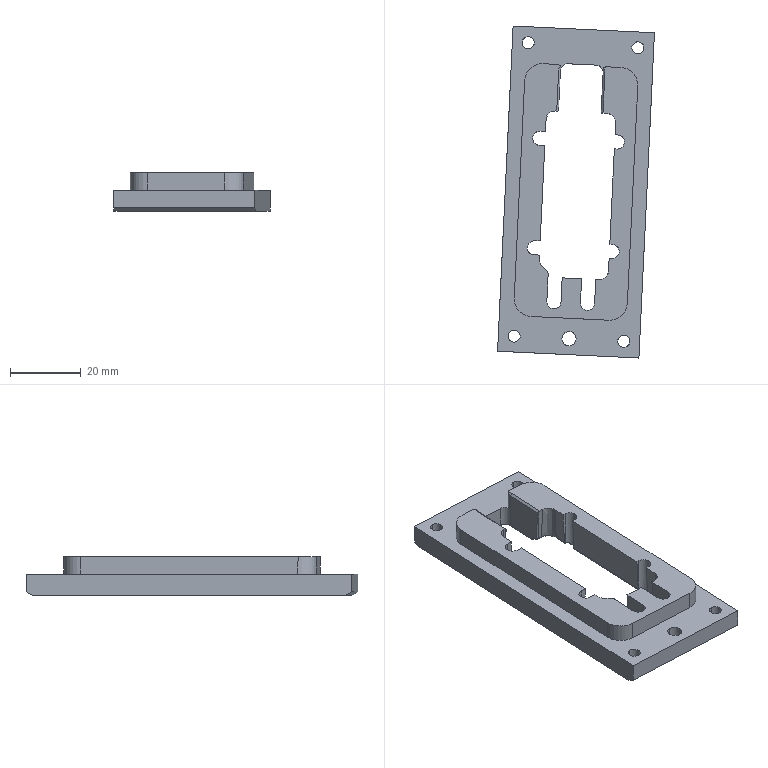Part | STEP file | X77-02201a | 1 solid | 275 faces | box 44.351 x 93.807 x 11.019 mm | volume 18832 mm3 | cylinder 119 | plane 79 | spline 69 | torus 3 | cone 3 | sphere 2 | commonest cylinder face diameters 1 x41 0.4 x26 4 x22 3.4 x8 6 x8 10 x5